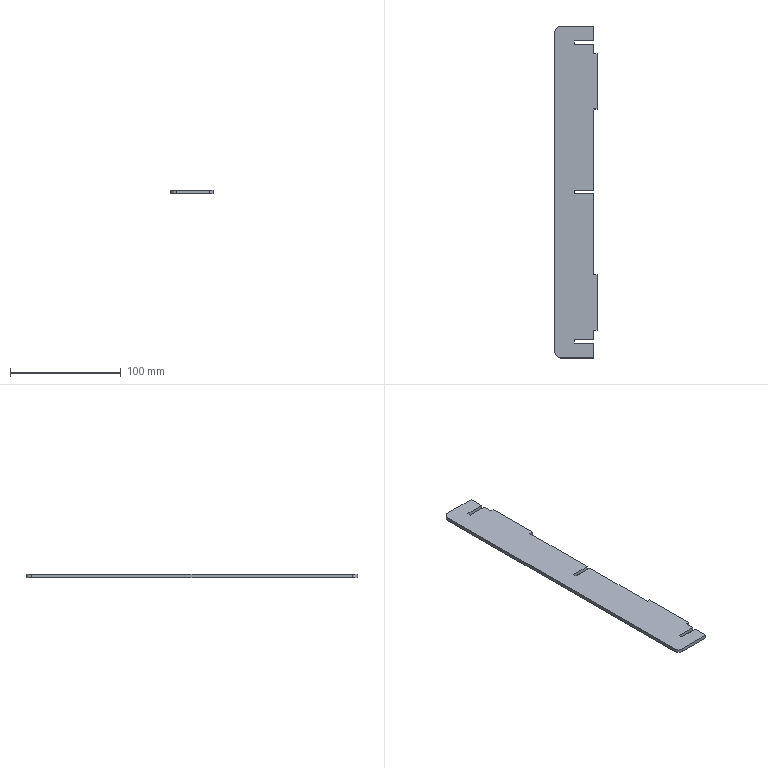Part | SolidWorks | features FlatPattern 1, SMBaseFlange 1, SheetMetal 1 | 1 solid | 28 faces | box 38 x 300 x 3.2 mm | volume 33985 mm3 | plane 26 | cylinder 2 | commonest cylinder face diameters 10 x2
STEP:
#1=CARTESIAN_POINT('',(198.,134.67,0.));
#2=VERTEX_POINT('',#1);
#3=CARTESIAN_POINT('',(198.,148.07,0.));
#4=VERTEX_POINT('',#3);
#5=CARTESIAN_POINT('',(198.,148.07,0.));
#6=DIRECTION('',(0.,1.,0.));
#7=VECTOR('',#6,1000.);
#8=LINE('',#5,#7);
#9=EDGE_CURVE('',#2,#4,#8,.T.);
#10=ORIENTED_EDGE('',*,*,#9,.F.);
#11=CARTESIAN_POINT('',(198.,134.67,-3.2));
#12=VERTEX_POINT('',#11);
#13=CARTESIAN_POINT('',(198.,134.67,-3.2));
#14=DIRECTION('',(0.,0.,1.));
#15=VECTOR('',#14,1000.);
#16=LINE('',#13,#15);
#17=EDGE_CURVE('',#12,#2,#16,.T.);
#18=ORIENTED_EDGE('',*,*,#17,.F.);
#19=CARTESIAN_POINT('',(198.,148.07,-3.2));
#20=VERTEX_POINT('',#19);
#21=CARTESIAN_POINT('',(198.,148.07,-3.2));
#22=DIRECTION('',(0.,1.,0.));
#23=VECTOR('',#22,1000.);
#24=LINE('',#21,#23);
#25=EDGE_CURVE('',#12,#20,#24,.T.);
#26=ORIENTED_EDGE('',*,*,#25,.T.);
#27=CARTESIAN_POINT('',(198.,148.07,-3.2));
#28=DIRECTION('',(0.,0.,1.));
#29=VECTOR('',#28,1000.);
#30=LINE('',#27,#29);
#31=EDGE_CURVE('',#20,#4,#30,.T.);
#32=ORIENTED_EDGE('',*,*,#31,.T.);
#33=EDGE_LOOP('',(#10,#18,#26,#32));
#34=FACE_OUTER_BOUND('',#33,.T.);
#35=CARTESIAN_POINT('',(198.,148.07,-3.2));
#36=DIRECTION('',(1.,0.,0.));
#37=DIRECTION('',(0.,1.,0.));
#38=AXIS2_PLACEMENT_3D('',#35,#36,#37);
#39=PLANE('',#38);
#40=ADVANCED_FACE('',(#34),#39,.T.);
#41=CARTESIAN_POINT('',(180.4,134.67,0.));
#42=VERTEX_POINT('',#41);
#43=CARTESIAN_POINT('',(198.,134.67,0.));
#44=DIRECTION('',(1.,0.,0.));
#45=VECTOR('',#44,1000.);
#46=LINE('',#43,#45);
#47=EDGE_CURVE('',#42,#2,#46,.T.);
#48=ORIENTED_EDGE('',*,*,#47,.F.);
#49=CARTESIAN_POINT('',(180.4,134.67,-3.2));
#50=VERTEX_POINT('',#49);
#51=CARTESIAN_POINT('',(180.4,134.67,-3.2));
#52=DIRECTION('',(0.,0.,1.));
#53=VECTOR('',#52,1000.);
#54=LINE('',#51,#53);
#55=EDGE_CURVE('',#50,#42,#54,.T.);
#56=ORIENTED_EDGE('',*,*,#55,.F.);
#57=CARTESIAN_POINT('',(198.,134.67,-3.2));
#58=DIRECTION('',(1.,0.,0.));
#59=VECTOR('',#58,1000.);
#60=LINE('',#57,#59);
#61=EDGE_CURVE('',#50,#12,#60,.T.);
#62=ORIENTED_EDGE('',*,*,#61,.T.);
#63=ORIENTED_EDGE('',*,*,#17,.T.);
#64=EDGE_LOOP('',(#48,#56,#62,#63));
#65=FACE_OUTER_BOUND('',#64,.T.);
#66=CARTESIAN_POINT('',(198.,134.67,-3.2));
#67=DIRECTION('',(0.,-1.,0.));
#68=DIRECTION('',(1.,0.,0.));
#69=AXIS2_PLACEMENT_3D('',#66,#67,#68);
#70=PLANE('',#69);
#71=ADVANCED_FACE('',(#65),#70,.T.);
#72=CARTESIAN_POINT('',(180.4,131.47,0.));
#73=VERTEX_POINT('',#72);
#74=CARTESIAN_POINT('',(180.4,134.67,0.));
#75=DIRECTION('',(0.,1.,0.));
#76=VECTOR('',#75,1000.);
#77=LINE('',#74,#76);
#78=EDGE_CURVE('',#73,#42,#77,.T.);
#79=ORIENTED_EDGE('',*,*,#78,.F.);
#80=CARTESIAN_POINT('',(180.4,131.47,-3.2));
#81=VERTEX_POINT('',#80);
#82=CARTESIAN_POINT('',(180.4,131.47,-3.2));
#83=DIRECTION('',(0.,0.,1.));
#84=VECTOR('',#83,1000.);
#85=LINE('',#82,#84);
#86=EDGE_CURVE('',#81,#73,#85,.T.);
#87=ORIENTED_EDGE('',*,*,#86,.F.);
#88=CARTESIAN_POINT('',(180.4,134.67,-3.2));
#89=DIRECTION('',(0.,1.,0.));
#90=VECTOR('',#89,1000.);
#91=LINE('',#88,#90);
#92=EDGE_CURVE('',#81,#50,#91,.T.);
#93=ORIENTED_EDGE('',*,*,#92,.T.);
#94=ORIENTED_EDGE('',*,*,#55,.T.);
#95=EDGE_LOOP('',(#79,#87,#93,#94));
#96=FACE_OUTER_BOUND('',#95,.T.);
#97=CARTESIAN_POINT('',(180.4,134.67,-3.2));
#98=DIRECTION('',(1.,0.,0.));
#99=DIRECTION('',(0.,0.,-1.));
#100=AXIS2_PLACEMENT_3D('',#97,#98,#99);
#101=PLANE('',#100);
#102=ADVANCED_FACE('',(#96),#101,.T.);
#103=CARTESIAN_POINT('',(198.,131.47,0.));
#104=VERTEX_POINT('',#103);
#105=CARTESIAN_POINT('',(180.4,131.47,0.));
#106=DIRECTION('',(-1.,0.,0.));
#107=VECTOR('',#106,1000.);
#108=LINE('',#105,#107);
#109=EDGE_CURVE('',#104,#73,#108,.T.);
#110=ORIENTED_EDGE('',*,*,#109,.F.);
#111=CARTESIAN_POINT('',(198.,131.47,-3.2));
#112=VERTEX_POINT('',#111);
#113=CARTESIAN_POINT('',(198.,131.47,-3.2));
#114=DIRECTION('',(0.,0.,1.));
#115=VECTOR('',#114,1000.);
#116=LINE('',#113,#115);
#117=EDGE_CURVE('',#112,#104,#116,.T.);
#118=ORIENTED_EDGE('',*,*,#117,.F.);
#119=CARTESIAN_POINT('',(180.4,131.47,-3.2));
#120=DIRECTION('',(-1.,0.,0.));
#121=VECTOR('',#120,1000.);
#122=LINE('',#119,#121);
#123=EDGE_CURVE('',#112,#81,#122,.T.);
#124=ORIENTED_EDGE('',*,*,#123,.T.);
#125=ORIENTED_EDGE('',*,*,#86,.T.);
#126=EDGE_LOOP('',(#110,#118,#124,#125));
#127=FACE_OUTER_BOUND('',#126,.T.);
#128=CARTESIAN_POINT('',(180.4,131.47,-3.2));
#129=DIRECTION('',(0.,1.,0.));
#130=DIRECTION('',(0.,0.,1.));
#131=AXIS2_PLACEMENT_3D('',#128,#129,#130);
#132=PLANE('',#131);
#133=ADVANCED_FACE('',(#127),#132,.T.);
#134=CARTESIAN_POINT('',(198.,123.07,0.));
#135=VERTEX_POINT('',#134);
#136=CARTESIAN_POINT('',(198.,131.47,0.));
#137=DIRECTION('',(0.,1.,0.));
#138=VECTOR('',#137,1000.);
#139=LINE('',#136,#138);
#140=EDGE_CURVE('',#135,#104,#139,.T.);
#141=ORIENTED_EDGE('',*,*,#140,.F.);
#142=CARTESIAN_POINT('',(198.,123.07,-3.2));
#143=VERTEX_POINT('',#142);
#144=CARTESIAN_POINT('',(198.,123.07,-3.2));
#145=DIRECTION('',(0.,0.,1.));
#146=VECTOR('',#145,1000.);
#147=LINE('',#144,#146);
#148=EDGE_CURVE('',#143,#135,#147,.T.);
#149=ORIENTED_EDGE('',*,*,#148,.F.);
#150=CARTESIAN_POINT('',(198.,131.47,-3.2));
#151=DIRECTION('',(0.,1.,0.));
#152=VECTOR('',#151,1000.);
#153=LINE('',#150,#152);
#154=EDGE_CURVE('',#143,#112,#153,.T.);
#155=ORIENTED_EDGE('',*,*,#154,.T.);
#156=ORIENTED_EDGE('',*,*,#117,.T.);
#157=EDGE_LOOP('',(#141,#149,#155,#156));
#158=FACE_OUTER_BOUND('',#157,.T.);
#159=CARTESIAN_POINT('',(198.,131.47,-3.2));
#160=DIRECTION('',(1.,0.,0.));
#161=DIRECTION('',(0.,1.,0.));
#162=AXIS2_PLACEMENT_3D('',#159,#160,#161);
#163=PLANE('',#162);
#164=ADVANCED_FACE('',(#158),#163,.T.);
#165=CARTESIAN_POINT('',(201.,123.07,0.));
#166=VERTEX_POINT('',#165);
#167=CARTESIAN_POINT('',(198.,123.07,0.));
#168=DIRECTION('',(-1.,0.,0.));
#169=VECTOR('',#168,1000.);
#170=LINE('',#167,#169);
#171=EDGE_CURVE('',#166,#135,#170,.T.);
#172=ORIENTED_EDGE('',*,*,#171,.F.);
#173=CARTESIAN_POINT('',(201.,123.07,-3.2));
#174=VERTEX_POINT('',#173);
#175=CARTESIAN_POINT('',(201.,123.07,-3.2));
#176=DIRECTION('',(0.,0.,1.));
#177=VECTOR('',#176,1000.);
#178=LINE('',#175,#177);
#179=EDGE_CURVE('',#174,#166,#178,.T.);
#180=ORIENTED_EDGE('',*,*,#179,.F.);
#181=CARTESIAN_POINT('',(198.,123.07,-3.2));
#182=DIRECTION('',(-1.,0.,0.));
#183=VECTOR('',#182,1000.);
#184=LINE('',#181,#183);
#185=EDGE_CURVE('',#174,#143,#184,.T.);
#186=ORIENTED_EDGE('',*,*,#185,.T.);
#187=ORIENTED_EDGE('',*,*,#148,.T.);
#188=EDGE_LOOP('',(#172,#180,#186,#187));
#189=FACE_OUTER_BOUND('',#188,.T.);
#190=CARTESIAN_POINT('',(198.,123.07,-3.2));
#191=DIRECTION('',(0.,1.,0.));
#192=DIRECTION('',(0.,0.,1.));
#193=AXIS2_PLACEMENT_3D('',#190,#191,#192);
#194=PLANE('',#193);
#195=ADVANCED_FACE('',(#189),#194,.T.);
#196=CARTESIAN_POINT('',(201.,73.07,0.));
#197=VERTEX_POINT('',#196);
#198=CARTESIAN_POINT('',(201.,123.07,0.));
#199=DIRECTION('',(0.,1.,0.));
#200=VECTOR('',#199,1000.);
#201=LINE('',#198,#200);
#202=EDGE_CURVE('',#197,#166,#201,.T.);
#203=ORIENTED_EDGE('',*,*,#202,.F.);
#204=CARTESIAN_POINT('',(201.,73.07,-3.2));
#205=VERTEX_POINT('',#204);
#206=CARTESIAN_POINT('',(201.,73.07,-3.2));
#207=DIRECTION('',(0.,0.,1.));
#208=VECTOR('',#207,1000.);
#209=LINE('',#206,#208);
#210=EDGE_CURVE('',#205,#197,#209,.T.);
#211=ORIENTED_EDGE('',*,*,#210,.F.);
#212=CARTESIAN_POINT('',(201.,123.07,-3.2));
#213=DIRECTION('',(0.,1.,0.));
#214=VECTOR('',#213,1000.);
#215=LINE('',#212,#214);
#216=EDGE_CURVE('',#205,#174,#215,.T.);
#217=ORIENTED_EDGE('',*,*,#216,.T.);
#218=ORIENTED_EDGE('',*,*,#179,.T.);
#219=EDGE_LOOP('',(#203,#211,#217,#218));
#220=FACE_OUTER_BOUND('',#219,.T.);
#221=CARTESIAN_POINT('',(201.,123.07,-3.2));
#222=DIRECTION('',(1.,0.,0.));
#223=DIRECTION('',(0.,0.,-1.));
#224=AXIS2_PLACEMENT_3D('',#221,#222,#223);
#225=PLANE('',#224);
#226=ADVANCED_FACE('',(#220),#225,.T.);
#227=CARTESIAN_POINT('',(198.,73.07,0.));
#228=VERTEX_POINT('',#227);
#229=CARTESIAN_POINT('',(201.,73.07,0.));
#230=DIRECTION('',(1.,0.,0.));
#231=VECTOR('',#230,1000.);
#232=LINE('',#229,#231);
#233=EDGE_CURVE('',#228,#197,#232,.T.);
#234=ORIENTED_EDGE('',*,*,#233,.F.);
#235=CARTESIAN_POINT('',(198.,73.07,-3.2));
#236=VERTEX_POINT('',#235);
#237=CARTESIAN_POINT('',(198.,73.07,-3.2));
#238=DIRECTION('',(0.,0.,1.));
#239=VECTOR('',#238,1000.);
#240=LINE('',#237,#239);
#241=EDGE_CURVE('',#236,#228,#240,.T.);
#242=ORIENTED_EDGE('',*,*,#241,.F.);
#243=CARTESIAN_POINT('',(201.,73.07,-3.2));
#244=DIRECTION('',(1.,0.,0.));
#245=VECTOR('',#244,1000.);
#246=LINE('',#243,#245);
#247=EDGE_CURVE('',#236,#205,#246,.T.);
#248=ORIENTED_EDGE('',*,*,#247,.T.);
#249=ORIENTED_EDGE('',*,*,#210,.T.);
#250=EDGE_LOOP('',(#234,#242,#248,#249));
#251=FACE_OUTER_BOUND('',#250,.T.);
#252=CARTESIAN_POINT('',(201.,73.07,-3.2));
#253=DIRECTION('',(0.,-1.,0.));
#254=DIRECTION('',(0.,0.,-1.));
#255=AXIS2_PLACEMENT_3D('',#252,#253,#254);
#256=PLANE('',#255);
#257=ADVANCED_FACE('',(#251),#256,.T.);
#258=CARTESIAN_POINT('',(198.,-0.3299,0.));
#259=VERTEX_POINT('',#258);
#260=CARTESIAN_POINT('',(198.,73.07,0.));
#261=DIRECTION('',(0.,1.,0.));
#262=VECTOR('',#261,1000.);
#263=LINE('',#260,#262);
#264=EDGE_CURVE('',#259,#228,#263,.T.);
#265=ORIENTED_EDGE('',*,*,#264,.F.);
#266=CARTESIAN_POINT('',(198.,-0.3299,-3.2));
#267=VERTEX_POINT('',#266);
#268=CARTESIAN_POINT('',(198.,-0.3299,-3.2));
#269=DIRECTION('',(0.,0.,1.));
#270=VECTOR('',#269,1000.);
#271=LINE('',#268,#270);
#272=EDGE_CURVE('',#267,#259,#271,.T.);
#273=ORIENTED_EDGE('',*,*,#272,.F.);
#274=CARTESIAN_POINT('',(198.,73.07,-3.2));
#275=DIRECTION('',(0.,1.,0.));
#276=VECTOR('',#275,1000.);
#277=LINE('',#274,#276);
#278=EDGE_CURVE('',#267,#236,#277,.T.);
#279=ORIENTED_EDGE('',*,*,#278,.T.);
#280=ORIENTED_EDGE('',*,*,#241,.T.);
#281=EDGE_LOOP('',(#265,#273,#279,#280));
#282=FACE_OUTER_BOUND('',#281,.T.);
#283=CARTESIAN_POINT('',(198.,73.07,-3.2));
#284=DIRECTION('',(1.,0.,0.));
#285=DIRECTION('',(0.,1.,0.));
#286=AXIS2_PLACEMENT_3D('',#283,#284,#285);
#287=PLANE('',#286);
#288=ADVANCED_FACE('',(#282),#287,.T.);
#289=CARTESIAN_POINT('',(180.4,-0.3299,0.));
#290=VERTEX_POINT('',#289);
#291=CARTESIAN_POINT('',(198.,-0.3299,0.));
#292=DIRECTION('',(1.,0.,0.));
#293=VECTOR('',#292,1000.);
#294=LINE('',#291,#293);
#295=EDGE_CURVE('',#290,#259,#294,.T.);
#296=ORIENTED_EDGE('',*,*,#295,.F.);
#297=CARTESIAN_POINT('',(180.4,-0.3299,-3.2));
#298=VERTEX_POINT('',#297);
#299=CARTESIAN_POINT('',(180.4,-0.3299,-3.2));
#300=DIRECTION('',(0.,0.,1.));
#301=VECTOR('',#300,1000.);
#302=LINE('',#299,#301);
#303=EDGE_CURVE('',#298,#290,#302,.T.);
#304=ORIENTED_EDGE('',*,*,#303,.F.);
#305=CARTESIAN_POINT('',(198.,-0.3299,-3.2));
#306=DIRECTION('',(1.,0.,0.));
#307=VECTOR('',#306,1000.);
#308=LINE('',#305,#307);
#309=EDGE_CURVE('',#298,#267,#308,.T.);
#310=ORIENTED_EDGE('',*,*,#309,.T.);
#311=ORIENTED_EDGE('',*,*,#272,.T.);
#312=EDGE_LOOP('',(#296,#304,#310,#311));
#313=FACE_OUTER_BOUND('',#312,.T.);
#314=CARTESIAN_POINT('',(198.,-0.3299,-3.2));
#315=DIRECTION('',(0.,-1.,0.));
#316=DIRECTION('',(0.,0.,-1.));
#317=AXIS2_PLACEMENT_3D('',#314,#315,#316);
#318=PLANE('',#317);
#319=ADVANCED_FACE('',(#313),#318,.T.);
#320=CARTESIAN_POINT('',(180.4,-3.53,0.));
#321=VERTEX_POINT('',#320);
#322=CARTESIAN_POINT('',(180.4,-0.3299,0.));
#323=DIRECTION('',(0.,1.,0.));
#324=VECTOR('',#323,1000.);
#325=LINE('',#322,#324);
#326=EDGE_CURVE('',#321,#290,#325,.T.);
#327=ORIENTED_EDGE('',*,*,#326,.F.);
#328=CARTESIAN_POINT('',(180.4,-3.53,-3.2));
#329=VERTEX_POINT('',#328);
#330=CARTESIAN_POINT('',(180.4,-3.53,-3.2));
#331=DIRECTION('',(0.,0.,1.));
#332=VECTOR('',#331,1000.);
#333=LINE('',#330,#332);
#334=EDGE_CURVE('',#329,#321,#333,.T.);
#335=ORIENTED_EDGE('',*,*,#334,.F.);
#336=CARTESIAN_POINT('',(180.4,-0.3299,-3.2));
#337=DIRECTION('',(0.,1.,0.));
#338=VECTOR('',#337,1000.);
#339=LINE('',#336,#338);
#340=EDGE_CURVE('',#329,#298,#339,.T.);
#341=ORIENTED_EDGE('',*,*,#340,.T.);
#342=ORIENTED_EDGE('',*,*,#303,.T.);
#343=EDGE_LOOP('',(#327,#335,#341,#342));
#344=FACE_OUTER_BOUND('',#343,.T.);
#345=CARTESIAN_POINT('',(180.4,-0.3299,-3.2));
#346=DIRECTION('',(1.,0.,0.));
#347=DIRECTION('',(0.,0.,-1.));
#348=AXIS2_PLACEMENT_3D('',#345,#346,#347);
#349=PLANE('',#348);
#350=ADVANCED_FACE('',(#344),#349,.T.);
#351=CARTESIAN_POINT('',(198.,-3.53,0.));
#352=VERTEX_POINT('',#351);
#353=CARTESIAN_POINT('',(180.4,-3.53,0.));
#354=DIRECTION('',(-1.,0.,0.));
#355=VECTOR('',#354,1000.);
#356=LINE('',#353,#355);
#357=EDGE_CURVE('',#352,#321,#356,.T.);
#358=ORIENTED_EDGE('',*,*,#357,.F.);
#359=CARTESIAN_POINT('',(198.,-3.53,-3.2));
#360=VERTEX_POINT('',#359);
#361=CARTESIAN_POINT('',(198.,-3.53,-3.2));
#362=DIRECTION('',(0.,0.,1.));
#363=VECTOR('',#362,1000.);
#364=LINE('',#361,#363);
#365=EDGE_CURVE('',#360,#352,#364,.T.);
#366=ORIENTED_EDGE('',*,*,#365,.F.);
#367=CARTESIAN_POINT('',(180.4,-3.53,-3.2));
#368=DIRECTION('',(-1.,0.,0.));
#369=VECTOR('',#368,1000.);
#370=LINE('',#367,#369);
#371=EDGE_CURVE('',#360,#329,#370,.T.);
#372=ORIENTED_EDGE('',*,*,#371,.T.);
#373=ORIENTED_EDGE('',*,*,#334,.T.);
#374=EDGE_LOOP('',(#358,#366,#372,#373));
#375=FACE_OUTER_BOUND('',#374,.T.);
#376=CARTESIAN_POINT('',(180.4,-3.53,-3.2));
#377=DIRECTION('',(0.,1.,0.));
#378=DIRECTION('',(0.,0.,1.));
#379=AXIS2_PLACEMENT_3D('',#376,#377,#378);
#380=PLANE('',#379);
#381=ADVANCED_FACE('',(#375),#380,.T.);
#382=CARTESIAN_POINT('',(198.,-76.93,0.));
#383=VERTEX_POINT('',#382);
#384=CARTESIAN_POINT('',(198.,-3.53,0.));
#385=DIRECTION('',(0.,1.,0.));
#386=VECTOR('',#385,1000.);
#387=LINE('',#384,#386);
#388=EDGE_CURVE('',#383,#352,#387,.T.);
#389=ORIENTED_EDGE('',*,*,#388,.F.);
#390=CARTESIAN_POINT('',(198.,-76.93,-3.2));
#391=VERTEX_POINT('',#390);
#392=CARTESIAN_POINT('',(198.,-76.93,-3.2));
#393=DIRECTION('',(0.,0.,1.));
#394=VECTOR('',#393,1000.);
#395=LINE('',#392,#394);
#396=EDGE_CURVE('',#391,#383,#395,.T.);
#397=ORIENTED_EDGE('',*,*,#396,.F.);
#398=CARTESIAN_POINT('',(198.,-3.53,-3.2));
#399=DIRECTION('',(0.,1.,0.));
#400=VECTOR('',#399,1000.);
#401=LINE('',#398,#400);
#402=EDGE_CURVE('',#391,#360,#401,.T.);
#403=ORIENTED_EDGE('',*,*,#402,.T.);
#404=ORIENTED_EDGE('',*,*,#365,.T.);
#405=EDGE_LOOP('',(#389,#397,#403,#404));
#406=FACE_OUTER_BOUND('',#405,.T.);
#407=CARTESIAN_POINT('',(198.,-3.53,-3.2));
#408=DIRECTION('',(1.,0.,0.));
#409=DIRECTION('',(0.,1.,0.));
#410=AXIS2_PLACEMENT_3D('',#407,#408,#409);
#411=PLANE('',#410);
#412=ADVANCED_FACE('',(#406),#411,.T.);
#413=CARTESIAN_POINT('',(201.,-76.93,0.));
#414=VERTEX_POINT('',#413);
#415=CARTESIAN_POINT('',(198.,-76.93,0.));
#416=DIRECTION('',(-1.,0.,0.));
#417=VECTOR('',#416,1000.);
#418=LINE('',#415,#417);
#419=EDGE_CURVE('',#414,#383,#418,.T.);
#420=ORIENTED_EDGE('',*,*,#419,.F.);
#421=CARTESIAN_POINT('',(201.,-76.93,-3.2));
#422=VERTEX_POINT('',#421);
#423=CARTESIAN_POINT('',(201.,-76.93,-3.2));
#424=DIRECTION('',(0.,0.,1.));
#425=VECTOR('',#424,1000.);
#426=LINE('',#423,#425);
#427=EDGE_CURVE('',#422,#414,#426,.T.);
#428=ORIENTED_EDGE('',*,*,#427,.F.);
#429=CARTESIAN_POINT('',(198.,-76.93,-3.2));
#430=DIRECTION('',(-1.,0.,0.));
#431=VECTOR('',#430,1000.);
#432=LINE('',#429,#431);
#433=EDGE_CURVE('',#422,#391,#432,.T.);
#434=ORIENTED_EDGE('',*,*,#433,.T.);
#435=ORIENTED_EDGE('',*,*,#396,.T.);
#436=EDGE_LOOP('',(#420,#428,#434,#435));
#437=FACE_OUTER_BOUND('',#436,.T.);
#438=CARTESIAN_POINT('',(198.,-76.93,-3.2));
#439=DIRECTION('',(0.,1.,0.));
#440=DIRECTION('',(-1.,0.,0.));
#441=AXIS2_PLACEMENT_3D('',#438,#439,#440);
#442=PLANE('',#441);
#443=ADVANCED_FACE('',(#437),#442,.T.);
#444=CARTESIAN_POINT('',(201.,-126.93,0.));
#445=VERTEX_POINT('',#444);
#446=CARTESIAN_POINT('',(201.,-76.93,0.));
#447=DIRECTION('',(0.,1.,0.));
#448=VECTOR('',#447,1000.);
#449=LINE('',#446,#448);
#450=EDGE_CURVE('',#445,#414,#449,.T.);
#451=ORIENTED_EDGE('',*,*,#450,.F.);
#452=CARTESIAN_POINT('',(201.,-126.93,-3.2));
#453=VERTEX_POINT('',#452);
#454=CARTESIAN_POINT('',(201.,-126.93,-3.2));
#455=DIRECTION('',(0.,0.,1.));
#456=VECTOR('',#455,1000.);
#457=LINE('',#454,#456);
#458=EDGE_CURVE('',#453,#445,#457,.T.);
#459=ORIENTED_EDGE('',*,*,#458,.F.);
#460=CARTESIAN_POINT('',(201.,-76.93,-3.2));
#461=DIRECTION('',(0.,1.,0.));
#462=VECTOR('',#461,1000.);
#463=LINE('',#460,#462);
#464=EDGE_CURVE('',#453,#422,#463,.T.);
#465=ORIENTED_EDGE('',*,*,#464,.T.);
#466=ORIENTED_EDGE('',*,*,#427,.T.);
#467=EDGE_LOOP('',(#451,#459,#465,#466));
#468=FACE_OUTER_BOUND('',#467,.T.);
#469=CARTESIAN_POINT('',(201.,-76.93,-3.2));
#470=DIRECTION('',(1.,0.,0.));
#471=DIRECTION('',(0.,1.,0.));
#472=AXIS2_PLACEMENT_3D('',#469,#470,#471);
#473=PLANE('',#472);
#474=ADVANCED_FACE('',(#468),#473,.T.);
#475=CARTESIAN_POINT('',(198.,-126.93,0.));
#476=VERTEX_POINT('',#475);
#477=CARTESIAN_POINT('',(201.,-126.93,0.));
#478=DIRECTION('',(1.,0.,0.));
#479=VECTOR('',#478,1000.);
#480=LINE('',#477,#479);
#481=EDGE_CURVE('',#476,#445,#480,.T.);
#482=ORIENTED_EDGE('',*,*,#481,.F.);
#483=CARTESIAN_POINT('',(198.,-126.93,-3.2));
#484=VERTEX_POINT('',#483);
#485=CARTESIAN_POINT('',(198.,-126.93,-3.2));
#486=DIRECTION('',(0.,0.,1.));
#487=VECTOR('',#486,1000.);
#488=LINE('',#485,#487);
#489=EDGE_CURVE('',#484,#476,#488,.T.);
#490=ORIENTED_EDGE('',*,*,#489,.F.);
#491=CARTESIAN_POINT('',(201.,-126.93,-3.2));
#492=DIRECTION('',(1.,0.,0.));
#493=VECTOR('',#492,1000.);
#494=LINE('',#491,#493);
#495=EDGE_CURVE('',#484,#453,#494,.T.);
#496=ORIENTED_EDGE('',*,*,#495,.T.);
#497=ORIENTED_EDGE('',*,*,#458,.T.);
#498=EDGE_LOOP('',(#482,#490,#496,#497));
#499=FACE_OUTER_BOUND('',#498,.T.);
#500=CARTESIAN_POINT('',(201.,-126.93,-3.2));
#501=DIRECTION('',(0.,-1.,0.));
#502=DIRECTION('',(0.,0.,-1.));
#503=AXIS2_PLACEMENT_3D('',#500,#501,#502);
#504=PLANE('',#503);
#505=ADVANCED_FACE('',(#499),#504,.T.);
#506=CARTESIAN_POINT('',(198.,-135.33,0.));
#507=VERTEX_POINT('',#506);
#508=CARTESIAN_POINT('',(198.,-126.93,0.));
#509=DIRECTION('',(0.,1.,0.));
#510=VECTOR('',#509,1000.);
#511=LINE('',#508,#510);
#512=EDGE_CURVE('',#507,#476,#511,.T.);
#513=ORIENTED_EDGE('',*,*,#512,.F.);
#514=CARTESIAN_POINT('',(198.,-135.33,-3.2));
#515=VERTEX_POINT('',#514);
#516=CARTESIAN_POINT('',(198.,-135.33,-3.2));
#517=DIRECTION('',(0.,0.,1.));
#518=VECTOR('',#517,1000.);
#519=LINE('',#516,#518);
#520=EDGE_CURVE('',#515,#507,#519,.T.);
#521=ORIENTED_EDGE('',*,*,#520,.F.);
#522=CARTESIAN_POINT('',(198.,-126.93,-3.2));
#523=DIRECTION('',(0.,1.,0.));
#524=VECTOR('',#523,1000.);
#525=LINE('',#522,#524);
#526=EDGE_CURVE('',#515,#484,#525,.T.);
#527=ORIENTED_EDGE('',*,*,#526,.T.);
#528=ORIENTED_EDGE('',*,*,#489,.T.);
#529=EDGE_LOOP('',(#513,#521,#527,#528));
#530=FACE_OUTER_BOUND('',#529,.T.);
#531=CARTESIAN_POINT('',(198.,-126.93,-3.2));
#532=DIRECTION('',(1.,0.,0.));
#533=DIRECTION('',(0.,1.,0.));
#534=AXIS2_PLACEMENT_3D('',#531,#532,#533);
#535=PLANE('',#534);
#536=ADVANCED_FACE('',(#530),#535,.T.);
#537=CARTESIAN_POINT('',(180.4,-135.33,0.));
#538=VERTEX_POINT('',#537);
#539=CARTESIAN_POINT('',(198.,-135.33,0.));
#540=DIRECTION('',(1.,0.,0.));
#541=VECTOR('',#540,1000.);
#542=LINE('',#539,#541);
#543=EDGE_CURVE('',#538,#507,#542,.T.);
#544=ORIENTED_EDGE('',*,*,#543,.F.);
#545=CARTESIAN_POINT('',(180.4,-135.33,-3.2));
#546=VERTEX_POINT('',#545);
#547=CARTESIAN_POINT('',(180.4,-135.33,-3.2));
#548=DIRECTION('',(0.,0.,1.));
#549=VECTOR('',#548,1000.);
#550=LINE('',#547,#549);
#551=EDGE_CURVE('',#546,#538,#550,.T.);
#552=ORIENTED_EDGE('',*,*,#551,.F.);
#553=CARTESIAN_POINT('',(198.,-135.33,-3.2));
#554=DIRECTION('',(1.,0.,0.));
#555=VECTOR('',#554,1000.);
#556=LINE('',#553,#555);
#557=EDGE_CURVE('',#546,#515,#556,.T.);
#558=ORIENTED_EDGE('',*,*,#557,.T.);
#559=ORIENTED_EDGE('',*,*,#520,.T.);
#560=EDGE_LOOP('',(#544,#552,#558,#559));
#561=FACE_OUTER_BOUND('',#560,.T.);
#562=CARTESIAN_POINT('',(198.,-135.33,-3.2));
#563=DIRECTION('',(0.,-1.,0.));
#564=DIRECTION('',(1.,0.,0.));
#565=AXIS2_PLACEMENT_3D('',#562,#563,#564);
#566=PLANE('',#565);
#567=ADVANCED_FACE('',(#561),#566,.T.);
#568=CARTESIAN_POINT('',(180.4,-138.53,0.));
#569=VERTEX_POINT('',#568);
#570=CARTESIAN_POINT('',(180.4,-135.33,0.));
#571=DIRECTION('',(0.,1.,0.));
#572=VECTOR('',#571,1000.);
#573=LINE('',#570,#572);
#574=EDGE_CURVE('',#569,#538,#573,.T.);
#575=ORIENTED_EDGE('',*,*,#574,.F.);
#576=CARTESIAN_POINT('',(180.4,-138.53,-3.2));
#577=VERTEX_POINT('',#576);
#578=CARTESIAN_POINT('',(180.4,-138.53,-3.2));
#579=DIRECTION('',(0.,0.,1.));
#580=VECTOR('',#579,1000.);
#581=LINE('',#578,#580);
#582=EDGE_CURVE('',#577,#569,#581,.T.);
#583=ORIENTED_EDGE('',*,*,#582,.F.);
#584=CARTESIAN_POINT('',(180.4,-135.33,-3.2));
#585=DIRECTION('',(0.,1.,0.));
#586=VECTOR('',#585,1000.);
#587=LINE('',#584,#586);
#588=EDGE_CURVE('',#577,#546,#587,.T.);
#589=ORIENTED_EDGE('',*,*,#588,.T.);
#590=ORIENTED_EDGE('',*,*,#551,.T.);
#591=EDGE_LOOP('',(#575,#583,#589,#590));
#592=FACE_OUTER_BOUND('',#591,.T.);
#593=CARTESIAN_POINT('',(180.4,-135.33,-3.2));
#594=DIRECTION('',(1.,0.,0.));
#595=DIRECTION('',(0.,0.,-1.));
#596=AXIS2_PLACEMENT_3D('',#593,#594,#595);
#597=PLANE('',#596);
#598=ADVANCED_FACE('',(#592),#597,.T.);
#599=CARTESIAN_POINT('',(198.,-138.53,0.));
#600=VERTEX_POINT('',#599);
#601=CARTESIAN_POINT('',(180.4,-138.53,0.));
#602=DIRECTION('',(-1.,0.,0.));
#603=VECTOR('',#602,1000.);
#604=LINE('',#601,#603);
#605=EDGE_CURVE('',#600,#569,#604,.T.);
#606=ORIENTED_EDGE('',*,*,#605,.F.);
#607=CARTESIAN_POINT('',(198.,-138.53,-3.2));
#608=VERTEX_POINT('',#607);
#609=CARTESIAN_POINT('',(198.,-138.53,-3.2));
#610=DIRECTION('',(0.,0.,1.));
#611=VECTOR('',#610,1000.);
#612=LINE('',#609,#611);
#613=EDGE_CURVE('',#608,#600,#612,.T.);
#614=ORIENTED_EDGE('',*,*,#613,.F.);
#615=CARTESIAN_POINT('',(180.4,-138.53,-3.2));
#616=DIRECTION('',(-1.,0.,0.));
#617=VECTOR('',#616,1000.);
#618=LINE('',#615,#617);
#619=EDGE_CURVE('',#608,#577,#618,.T.);
#620=ORIENTED_EDGE('',*,*,#619,.T.);
#621=ORIENTED_EDGE('',*,*,#582,.T.);
#622=EDGE_LOOP('',(#606,#614,#620,#621));
#623=FACE_OUTER_BOUND('',#622,.T.);
#624=CARTESIAN_POINT('',(180.4,-138.53,-3.2));
#625=DIRECTION('',(0.,1.,0.));
#626=DIRECTION('',(0.,0.,1.));
#627=AXIS2_PLACEMENT_3D('',#624,#625,#626);
#628=PLANE('',#627);
#629=ADVANCED_FACE('',(#623),#628,.T.);
#630=CARTESIAN_POINT('',(198.,-151.93,0.));
#631=VERTEX_POINT('',#630);
#632=CARTESIAN_POINT('',(198.,-138.53,0.));
#633=DIRECTION('',(0.,1.,0.));
#634=VECTOR('',#633,1000.);
#635=LINE('',#632,#634);
#636=EDGE_CURVE('',#631,#600,#635,.T.);
#637=ORIENTED_EDGE('',*,*,#636,.F.);
#638=CARTESIAN_POINT('',(198.,-151.93,-3.2));
#639=VERTEX_POINT('',#638);
#640=CARTESIAN_POINT('',(198.,-151.93,-3.2));
#641=DIRECTION('',(0.,0.,1.));
#642=VECTOR('',#641,1000.);
#643=LINE('',#640,#642);
#644=EDGE_CURVE('',#639,#631,#643,.T.);
#645=ORIENTED_EDGE('',*,*,#644,.F.);
#646=CARTESIAN_POINT('',(198.,-138.53,-3.2));
#647=DIRECTION('',(0.,1.,0.));
#648=VECTOR('',#647,1000.);
#649=LINE('',#646,#648);
#650=EDGE_CURVE('',#639,#608,#649,.T.);
#651=ORIENTED_EDGE('',*,*,#650,.T.);
#652=ORIENTED_EDGE('',*,*,#613,.T.);
#653=EDGE_LOOP('',(#637,#645,#651,#652));
#654=FACE_OUTER_BOUND('',#653,.T.);
#655=CARTESIAN_POINT('',(198.,-138.53,-3.2));
#656=DIRECTION('',(1.,0.,0.));
#657=DIRECTION('',(0.,1.,0.));
#658=AXIS2_PLACEMENT_3D('',#655,#656,#657);
#659=PLANE('',#658);
#660=ADVANCED_FACE('',(#654),#659,.T.);
#661=CARTESIAN_POINT('',(168.,-151.93,0.));
#662=VERTEX_POINT('',#661);
#663=CARTESIAN_POINT('',(198.,-151.93,0.));
#664=DIRECTION('',(1.,0.,0.));
#665=VECTOR('',#664,1000.);
#666=LINE('',#663,#665);
#667=EDGE_CURVE('',#662,#631,#666,.T.);
#668=ORIENTED_EDGE('',*,*,#667,.F.);
#669=CARTESIAN_POINT('',(168.,-151.93,-3.2));
#670=VERTEX_POINT('',#669);
#671=CARTESIAN_POINT('',(168.,-151.93,-3.2));
#672=DIRECTION('',(0.,0.,1.));
#673=VECTOR('',#672,1000.);
#674=LINE('',#671,#673);
#675=EDGE_CURVE('',#670,#662,#674,.T.);
#676=ORIENTED_EDGE('',*,*,#675,.F.);
#677=CARTESIAN_POINT('',(198.,-151.93,-3.2));
#678=DIRECTION('',(1.,0.,0.));
#679=VECTOR('',#678,1000.);
#680=LINE('',#677,#679);
#681=EDGE_CURVE('',#670,#639,#680,.T.);
#682=ORIENTED_EDGE('',*,*,#681,.T.);
#683=ORIENTED_EDGE('',*,*,#644,.T.);
#684=EDGE_LOOP('',(#668,#676,#682,#683));
#685=FACE_OUTER_BOUND('',#684,.T.);
#686=CARTESIAN_POINT('',(198.,-151.93,-3.2));
#687=DIRECTION('',(0.,-1.,0.));
#688=DIRECTION('',(0.,0.,-1.));
#689=AXIS2_PLACEMENT_3D('',#686,#687,#688);
#690=PLANE('',#689);
#691=ADVANCED_FACE('',(#685),#690,.T.);
#692=CARTESIAN_POINT('',(163.,-146.93,0.));
#693=VERTEX_POINT('',#692);
#694=CARTESIAN_POINT('',(168.,-146.93,0.));
#695=DIRECTION('',(0.,0.,1.));
#696=DIRECTION('',(-1.,0.,0.));
#697=AXIS2_PLACEMENT_3D('',#694,#695,#696);
#698=CIRCLE('',#697,5.);
#699=EDGE_CURVE('',#693,#662,#698,.T.);
#700=ORIENTED_EDGE('',*,*,#699,.F.);
#701=CARTESIAN_POINT('',(163.,-146.93,-3.2));
#702=VERTEX_POINT('',#701);
#703=CARTESIAN_POINT('',(163.,-146.93,-3.2));
#704=DIRECTION('',(0.,0.,1.));
#705=VECTOR('',#704,1000.);
#706=LINE('',#703,#705);
#707=EDGE_CURVE('',#702,#693,#706,.T.);
#708=ORIENTED_EDGE('',*,*,#707,.F.);
#709=CARTESIAN_POINT('',(168.,-146.93,-3.2));
#710=DIRECTION('',(0.,0.,1.));
#711=DIRECTION('',(-1.,0.,0.));
#712=AXIS2_PLACEMENT_3D('',#709,#710,#711);
#713=CIRCLE('',#712,5.);
#714=EDGE_CURVE('',#702,#670,#713,.T.);
#715=ORIENTED_EDGE('',*,*,#714,.T.);
#716=ORIENTED_EDGE('',*,*,#675,.T.);
#717=EDGE_LOOP('',(#700,#708,#715,#716));
#718=FACE_OUTER_BOUND('',#717,.T.);
#719=CARTESIAN_POINT('',(168.,-146.93,-3.2));
#720=DIRECTION('',(0.,0.,1.));
#721=DIRECTION('',(1.,0.,0.));
#722=AXIS2_PLACEMENT_3D('',#719,#720,#721);
#723=CYLINDRICAL_SURFACE('',#722,5.);
#724=ADVANCED_FACE('',(#718),#723,.T.);
#725=CARTESIAN_POINT('',(163.,143.07,0.));
#726=VERTEX_POINT('',#725);
#727=CARTESIAN_POINT('',(163.,143.07,0.));
#728=DIRECTION('',(0.,-1.,0.));
#729=VECTOR('',#728,1000.);
#730=LINE('',#727,#729);
#731=EDGE_CURVE('',#726,#693,#730,.T.);
#732=ORIENTED_EDGE('',*,*,#731,.F.);
#733=CARTESIAN_POINT('',(163.,143.07,-3.2));
#734=VERTEX_POINT('',#733);
#735=CARTESIAN_POINT('',(163.,143.07,-3.2));
#736=DIRECTION('',(0.,0.,1.));
#737=VECTOR('',#736,1000.);
#738=LINE('',#735,#737);
#739=EDGE_CURVE('',#734,#726,#738,.T.);
#740=ORIENTED_EDGE('',*,*,#739,.F.);
#741=CARTESIAN_POINT('',(163.,143.07,-3.2));
#742=DIRECTION('',(0.,-1.,0.));
#743=VECTOR('',#742,1000.);
#744=LINE('',#741,#743);
#745=EDGE_CURVE('',#734,#702,#744,.T.);
#746=ORIENTED_EDGE('',*,*,#745,.T.);
#747=ORIENTED_EDGE('',*,*,#707,.T.);
#748=EDGE_LOOP('',(#732,#740,#746,#747));
#749=FACE_OUTER_BOUND('',#748,.T.);
#750=CARTESIAN_POINT('',(163.,143.07,-3.2));
#751=DIRECTION('',(-1.,0.,0.));
#752=DIRECTION('',(0.,-1.,0.));
#753=AXIS2_PLACEMENT_3D('',#750,#751,#752);
#754=PLANE('',#753);
#755=ADVANCED_FACE('',(#749),#754,.T.);
#756=CARTESIAN_POINT('',(168.,148.07,0.));
#757=VERTEX_POINT('',#756);
#758=CARTESIAN_POINT('',(168.,143.07,0.));
#759=DIRECTION('',(0.,0.,1.));
#760=DIRECTION('',(1.,0.,0.));
#761=AXIS2_PLACEMENT_3D('',#758,#759,#760);
#762=CIRCLE('',#761,5.);
#763=EDGE_CURVE('',#757,#726,#762,.T.);
#764=ORIENTED_EDGE('',*,*,#763,.F.);
#765=CARTESIAN_POINT('',(168.,148.07,-3.2));
#766=VERTEX_POINT('',#765);
#767=CARTESIAN_POINT('',(168.,148.07,-3.2));
#768=DIRECTION('',(0.,0.,1.));
#769=VECTOR('',#768,1000.);
#770=LINE('',#767,#769);
#771=EDGE_CURVE('',#766,#757,#770,.T.);
#772=ORIENTED_EDGE('',*,*,#771,.F.);
#773=CARTESIAN_POINT('',(168.,143.07,-3.2));
#774=DIRECTION('',(0.,0.,1.));
#775=DIRECTION('',(1.,0.,0.));
#776=AXIS2_PLACEMENT_3D('',#773,#774,#775);
#777=CIRCLE('',#776,5.);
#778=EDGE_CURVE('',#766,#734,#777,.T.);
#779=ORIENTED_EDGE('',*,*,#778,.T.);
#780=ORIENTED_EDGE('',*,*,#739,.T.);
#781=EDGE_LOOP('',(#764,#772,#779,#780));
#782=FACE_OUTER_BOUND('',#781,.T.);
#783=CARTESIAN_POINT('',(168.,143.07,-3.2));
#784=DIRECTION('',(0.,0.,1.));
#785=DIRECTION('',(1.,0.,0.));
#786=AXIS2_PLACEMENT_3D('',#783,#784,#785);
#787=CYLINDRICAL_SURFACE('',#786,5.);
#788=ADVANCED_FACE('',(#782),#787,.T.);
#789=CARTESIAN_POINT('',(198.,148.07,0.));
#790=DIRECTION('',(-1.,0.,0.));
#791=VECTOR('',#790,1000.);
#792=LINE('',#789,#791);
#793=EDGE_CURVE('',#4,#757,#792,.T.);
#794=ORIENTED_EDGE('',*,*,#793,.F.);
#795=ORIENTED_EDGE('',*,*,#31,.F.);
#796=CARTESIAN_POINT('',(198.,148.07,-3.2));
#797=DIRECTION('',(-1.,0.,0.));
#798=VECTOR('',#797,1000.);
#799=LINE('',#796,#798);
#800=EDGE_CURVE('',#20,#766,#799,.T.);
#801=ORIENTED_EDGE('',*,*,#800,.T.);
#802=ORIENTED_EDGE('',*,*,#771,.T.);
#803=EDGE_LOOP('',(#794,#795,#801,#802));
#804=FACE_OUTER_BOUND('',#803,.T.);
#805=CARTESIAN_POINT('',(198.,148.07,-3.2));
#806=DIRECTION('',(0.,1.,0.));
#807=DIRECTION('',(-1.,0.,0.));
#808=AXIS2_PLACEMENT_3D('',#805,#806,#807);
#809=PLANE('',#808);
#810=ADVANCED_FACE('',(#804),#809,.T.);
#811=ORIENTED_EDGE('',*,*,#25,.F.);
#812=ORIENTED_EDGE('',*,*,#61,.F.);
#813=ORIENTED_EDGE('',*,*,#92,.F.);
#814=ORIENTED_EDGE('',*,*,#123,.F.);
#815=ORIENTED_EDGE('',*,*,#154,.F.);
#816=ORIENTED_EDGE('',*,*,#185,.F.);
#817=ORIENTED_EDGE('',*,*,#216,.F.);
#818=ORIENTED_EDGE('',*,*,#247,.F.);
#819=ORIENTED_EDGE('',*,*,#278,.F.);
#820=ORIENTED_EDGE('',*,*,#309,.F.);
#821=ORIENTED_EDGE('',*,*,#340,.F.);
#822=ORIENTED_EDGE('',*,*,#371,.F.);
#823=ORIENTED_EDGE('',*,*,#402,.F.);
#824=ORIENTED_EDGE('',*,*,#433,.F.);
#825=ORIENTED_EDGE('',*,*,#464,.F.);
#826=ORIENTED_EDGE('',*,*,#495,.F.);
#827=ORIENTED_EDGE('',*,*,#526,.F.);
#828=ORIENTED_EDGE('',*,*,#557,.F.);
#829=ORIENTED_EDGE('',*,*,#588,.F.);
#830=ORIENTED_EDGE('',*,*,#619,.F.);
#831=ORIENTED_EDGE('',*,*,#650,.F.);
#832=ORIENTED_EDGE('',*,*,#681,.F.);
#833=ORIENTED_EDGE('',*,*,#714,.F.);
#834=ORIENTED_EDGE('',*,*,#745,.F.);
#835=ORIENTED_EDGE('',*,*,#778,.F.);
#836=ORIENTED_EDGE('',*,*,#800,.F.);
#837=EDGE_LOOP('',(#811,#812,#813,#814,#815,#816,#817,#818,#819,#820,#821,#822,#823,#824,#825,#826,#827,#828,#829,#830,#831,#832,#833,#834,#835,#836));
#838=FACE_OUTER_BOUND('',#837,.T.);
#839=CARTESIAN_POINT('',(168.,-146.93,-3.2));
#840=DIRECTION('',(0.,0.,-1.));
#841=DIRECTION('',(-1.,0.,0.));
#842=AXIS2_PLACEMENT_3D('',#839,#840,#841);
#843=PLANE('',#842);
#844=ADVANCED_FACE('',(#838),#843,.T.);
#845=ORIENTED_EDGE('',*,*,#9,.T.);
#846=ORIENTED_EDGE('',*,*,#793,.T.);
#847=ORIENTED_EDGE('',*,*,#763,.T.);
#848=ORIENTED_EDGE('',*,*,#731,.T.);
#849=ORIENTED_EDGE('',*,*,#699,.T.);
#850=ORIENTED_EDGE('',*,*,#667,.T.);
#851=ORIENTED_EDGE('',*,*,#636,.T.);
#852=ORIENTED_EDGE('',*,*,#605,.T.);
#853=ORIENTED_EDGE('',*,*,#574,.T.);
#854=ORIENTED_EDGE('',*,*,#543,.T.);
#855=ORIENTED_EDGE('',*,*,#512,.T.);
#856=ORIENTED_EDGE('',*,*,#481,.T.);
#857=ORIENTED_EDGE('',*,*,#450,.T.);
#858=ORIENTED_EDGE('',*,*,#419,.T.);
#859=ORIENTED_EDGE('',*,*,#388,.T.);
#860=ORIENTED_EDGE('',*,*,#357,.T.);
#861=ORIENTED_EDGE('',*,*,#326,.T.);
#862=ORIENTED_EDGE('',*,*,#295,.T.);
#863=ORIENTED_EDGE('',*,*,#264,.T.);
#864=ORIENTED_EDGE('',*,*,#233,.T.);
#865=ORIENTED_EDGE('',*,*,#202,.T.);
#866=ORIENTED_EDGE('',*,*,#171,.T.);
#867=ORIENTED_EDGE('',*,*,#140,.T.);
#868=ORIENTED_EDGE('',*,*,#109,.T.);
#869=ORIENTED_EDGE('',*,*,#78,.T.);
#870=ORIENTED_EDGE('',*,*,#47,.T.);
#871=EDGE_LOOP('',(#845,#846,#847,#848,#849,#850,#851,#852,#853,#854,#855,#856,#857,#858,#859,#860,#861,#862,#863,#864,#865,#866,#867,#868,#869,#870));
#872=FACE_OUTER_BOUND('',#871,.T.);
#873=CARTESIAN_POINT('',(168.,-146.93,0.));
#874=DIRECTION('',(0.,0.,-1.));
#875=DIRECTION('',(-1.,0.,0.));
#876=AXIS2_PLACEMENT_3D('',#873,#874,#875);
#877=PLANE('',#876);
#878=ADVANCED_FACE('',(#872),#877,.F.);
#879=CLOSED_SHELL('',(#40,#71,#102,#133,#164,#195,#226,#257,#288,#319,#350,#381,#412,#443,#474,#505,#536,#567,#598,#629,#660,#691,#724,#755,#788,#810,#844,#878));
#880=MANIFOLD_SOLID_BREP('',#879);
#881=CARTESIAN_POINT('',(0.,0.,0.));
#882=DIRECTION('',(0.,0.,1.));
#883=DIRECTION('',(1.,0.,0.));
#884=AXIS2_PLACEMENT_3D('',#881,#882,#883);
#885=(LENGTH_UNIT()NAMED_UNIT(*)SI_UNIT(.MILLI.,.METRE.));
#886=UNCERTAINTY_MEASURE_WITH_UNIT(LENGTH_MEASURE(0.00001),#885,'','');
#887=(NAMED_UNIT(*)PLANE_ANGLE_UNIT()SI_UNIT($,.RADIAN.));
#888=(NAMED_UNIT(*)SI_UNIT($,.STERADIAN.)SOLID_ANGLE_UNIT());
#889=(GEOMETRIC_REPRESENTATION_CONTEXT(3)GLOBAL_UNCERTAINTY_ASSIGNED_CONTEXT((#886))GLOBAL_UNIT_ASSIGNED_CONTEXT((#885,#887,#888))REPRESENTATION_CONTEXT('',''));
#890=ADVANCED_BREP_SHAPE_REPRESENTATION('',(#880,#884),#889);